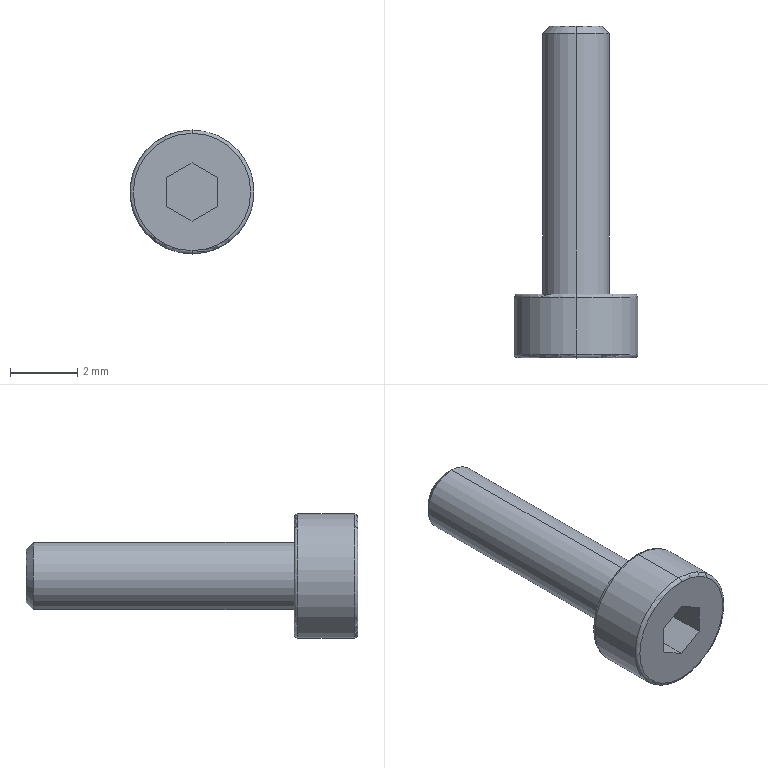Part | SolidWorks | features ICE 2, Extrusion 1, Fillet 1, StudWizard 1 | 1 solid | 20 faces | box 3.7 x 9.9 x 3.7 mm | volume 41.479 mm3 | plane 10 | torus 4 | cylinder 4 | cone 2 | commonest cylinder face diameters 2 x2 3.7 x2
STEP:
#1=CARTESIAN_POINT('',(0.,1.8,-1.85));
#2=VERTEX_POINT('',#1);
#3=CARTESIAN_POINT('',(0.,1.8,1.85));
#4=VERTEX_POINT('',#3);
#5=CARTESIAN_POINT('',(0.,1.8,0.));
#6=DIRECTION('',(0.,-1.,0.));
#7=DIRECTION('',(0.,0.,1.));
#8=AXIS2_PLACEMENT_3D('',#5,#6,#7);
#9=CIRCLE('',#8,1.85);
#10=EDGE_CURVE('',#2,#4,#9,.T.);
#11=ORIENTED_EDGE('',*,*,#10,.F.);
#12=CARTESIAN_POINT('',(0.,1.9,-1.75));
#13=VERTEX_POINT('',#12);
#14=CARTESIAN_POINT('',(0.,1.8,-1.75));
#15=DIRECTION('',(1.,0.,0.));
#16=DIRECTION('',(0.,0.,-1.));
#17=AXIS2_PLACEMENT_3D('',#14,#15,#16);
#18=CIRCLE('',#17,0.1);
#19=EDGE_CURVE('',#2,#13,#18,.T.);
#20=ORIENTED_EDGE('',*,*,#19,.T.);
#21=CARTESIAN_POINT('',(0.,1.9,1.75));
#22=VERTEX_POINT('',#21);
#23=CARTESIAN_POINT('',(0.,1.9,0.));
#24=DIRECTION('',(0.,1.,0.));
#25=DIRECTION('',(0.,0.,1.));
#26=AXIS2_PLACEMENT_3D('',#23,#24,#25);
#27=CIRCLE('',#26,1.75);
#28=EDGE_CURVE('',#22,#13,#27,.T.);
#29=ORIENTED_EDGE('',*,*,#28,.F.);
#30=CARTESIAN_POINT('',(0.,1.8,1.75));
#31=DIRECTION('',(-1.,0.,0.));
#32=DIRECTION('',(0.,0.,1.));
#33=AXIS2_PLACEMENT_3D('',#30,#31,#32);
#34=CIRCLE('',#33,0.1);
#35=EDGE_CURVE('',#4,#22,#34,.T.);
#36=ORIENTED_EDGE('',*,*,#35,.F.);
#37=EDGE_LOOP('',(#11,#20,#29,#36));
#38=FACE_OUTER_BOUND('',#37,.T.);
#39=CARTESIAN_POINT('',(0.,1.8,0.));
#40=DIRECTION('',(0.,1.,0.));
#41=DIRECTION('',(0.,0.,1.));
#42=AXIS2_PLACEMENT_3D('',#39,#40,#41);
#43=TOROIDAL_SURFACE('',#42,1.75,0.1);
#44=ADVANCED_FACE('',(#38),#43,.T.);
#45=CARTESIAN_POINT('',(0.,0.,-1.75));
#46=VERTEX_POINT('',#45);
#47=CARTESIAN_POINT('',(0.,0.,1.75));
#48=VERTEX_POINT('',#47);
#49=CARTESIAN_POINT('',(0.,0.,0.));
#50=DIRECTION('',(0.,-1.,0.));
#51=DIRECTION('',(0.,0.,1.));
#52=AXIS2_PLACEMENT_3D('',#49,#50,#51);
#53=CIRCLE('',#52,1.75);
#54=EDGE_CURVE('',#46,#48,#53,.T.);
#55=ORIENTED_EDGE('',*,*,#54,.F.);
#56=CARTESIAN_POINT('',(0.,0.1,-1.85));
#57=VERTEX_POINT('',#56);
#58=CARTESIAN_POINT('',(0.,0.1,-1.75));
#59=DIRECTION('',(1.,0.,0.));
#60=DIRECTION('',(0.,0.,-1.));
#61=AXIS2_PLACEMENT_3D('',#58,#59,#60);
#62=CIRCLE('',#61,0.1);
#63=EDGE_CURVE('',#46,#57,#62,.T.);
#64=ORIENTED_EDGE('',*,*,#63,.T.);
#65=CARTESIAN_POINT('',(0.,0.1,1.85));
#66=VERTEX_POINT('',#65);
#67=CARTESIAN_POINT('',(0.,0.1,0.));
#68=DIRECTION('',(0.,1.,0.));
#69=DIRECTION('',(0.,0.,1.));
#70=AXIS2_PLACEMENT_3D('',#67,#68,#69);
#71=CIRCLE('',#70,1.85);
#72=EDGE_CURVE('',#66,#57,#71,.T.);
#73=ORIENTED_EDGE('',*,*,#72,.F.);
#74=CARTESIAN_POINT('',(0.,0.1,1.75));
#75=DIRECTION('',(-1.,0.,0.));
#76=DIRECTION('',(0.,0.,1.));
#77=AXIS2_PLACEMENT_3D('',#74,#75,#76);
#78=CIRCLE('',#77,0.1);
#79=EDGE_CURVE('',#48,#66,#78,.T.);
#80=ORIENTED_EDGE('',*,*,#79,.F.);
#81=EDGE_LOOP('',(#55,#64,#73,#80));
#82=FACE_OUTER_BOUND('',#81,.T.);
#83=CARTESIAN_POINT('',(0.,0.1,0.));
#84=DIRECTION('',(0.,1.,0.));
#85=DIRECTION('',(0.,0.,1.));
#86=AXIS2_PLACEMENT_3D('',#83,#84,#85);
#87=TOROIDAL_SURFACE('',#86,1.75,0.1);
#88=ADVANCED_FACE('',(#82),#87,.T.);
#89=CARTESIAN_POINT('',(0.,9.9,-0.7835));
#90=VERTEX_POINT('',#89);
#91=CARTESIAN_POINT('',(0.,9.9,0.7835));
#92=VERTEX_POINT('',#91);
#93=CARTESIAN_POINT('',(0.,9.9,0.));
#94=DIRECTION('',(0.,-1.,0.));
#95=DIRECTION('',(0.,0.,-1.));
#96=AXIS2_PLACEMENT_3D('',#93,#94,#95);
#97=CIRCLE('',#96,0.7835);
#98=EDGE_CURVE('',#90,#92,#97,.T.);
#99=ORIENTED_EDGE('',*,*,#98,.T.);
#100=CARTESIAN_POINT('',(0.,9.684,1.));
#101=VERTEX_POINT('',#100);
#102=CARTESIAN_POINT('',(0.,9.684,1.));
#103=DIRECTION('',(0.,-0.7071,0.7071));
#104=VECTOR('',#103,1000.);
#105=LINE('',#102,#104);
#106=EDGE_CURVE('',#92,#101,#105,.T.);
#107=ORIENTED_EDGE('',*,*,#106,.T.);
#108=CARTESIAN_POINT('',(0.,9.684,-1.));
#109=VERTEX_POINT('',#108);
#110=CARTESIAN_POINT('',(0.,9.684,0.));
#111=DIRECTION('',(0.,-1.,0.));
#112=DIRECTION('',(0.,0.,-1.));
#113=AXIS2_PLACEMENT_3D('',#110,#111,#112);
#114=CIRCLE('',#113,1.);
#115=EDGE_CURVE('',#109,#101,#114,.T.);
#116=ORIENTED_EDGE('',*,*,#115,.F.);
#117=CARTESIAN_POINT('',(0.,9.684,-1.));
#118=DIRECTION('',(0.,-0.7071,-0.7071));
#119=VECTOR('',#118,1000.);
#120=LINE('',#117,#119);
#121=EDGE_CURVE('',#90,#109,#120,.T.);
#122=ORIENTED_EDGE('',*,*,#121,.F.);
#123=EDGE_LOOP('',(#99,#107,#116,#122));
#124=FACE_OUTER_BOUND('',#123,.T.);
#125=CARTESIAN_POINT('',(0.,9.684,0.));
#126=DIRECTION('',(0.,-1.,0.));
#127=DIRECTION('',(0.,0.,-1.));
#128=AXIS2_PLACEMENT_3D('',#125,#126,#127);
#129=CONICAL_SURFACE('',#128,1.,0.7854);
#130=ADVANCED_FACE('',(#124),#129,.T.);
#131=ORIENTED_EDGE('',*,*,#115,.T.);
#132=CARTESIAN_POINT('',(0.,1.9,1.));
#133=VERTEX_POINT('',#132);
#134=CARTESIAN_POINT('',(0.,6.72,1.));
#135=DIRECTION('',(0.,-1.,0.));
#136=VECTOR('',#135,1000.);
#137=LINE('',#134,#136);
#138=EDGE_CURVE('',#101,#133,#137,.T.);
#139=ORIENTED_EDGE('',*,*,#138,.T.);
#140=CARTESIAN_POINT('',(0.,1.9,-1.));
#141=VERTEX_POINT('',#140);
#142=CARTESIAN_POINT('',(0.,1.9,0.));
#143=DIRECTION('',(0.,1.,0.));
#144=DIRECTION('',(0.,0.,1.));
#145=AXIS2_PLACEMENT_3D('',#142,#143,#144);
#146=CIRCLE('',#145,1.);
#147=EDGE_CURVE('',#133,#141,#146,.T.);
#148=ORIENTED_EDGE('',*,*,#147,.T.);
#149=CARTESIAN_POINT('',(0.,6.72,-1.));
#150=DIRECTION('',(0.,-1.,0.));
#151=VECTOR('',#150,1000.);
#152=LINE('',#149,#151);
#153=EDGE_CURVE('',#109,#141,#152,.T.);
#154=ORIENTED_EDGE('',*,*,#153,.F.);
#155=EDGE_LOOP('',(#131,#139,#148,#154));
#156=FACE_OUTER_BOUND('',#155,.T.);
#157=CARTESIAN_POINT('',(0.,6.72,0.));
#158=DIRECTION('',(0.,-1.,0.));
#159=DIRECTION('',(0.,0.,-1.));
#160=AXIS2_PLACEMENT_3D('',#157,#158,#159);
#161=CYLINDRICAL_SURFACE('',#160,1.);
#162=ADVANCED_FACE('',(#156),#161,.T.);
#163=ORIENTED_EDGE('',*,*,#10,.T.);
#164=CARTESIAN_POINT('',(0.,1.9,1.85));
#165=DIRECTION('',(0.,-1.,0.));
#166=VECTOR('',#165,1000.);
#167=LINE('',#164,#166);
#168=EDGE_CURVE('',#4,#66,#167,.T.);
#169=ORIENTED_EDGE('',*,*,#168,.T.);
#170=ORIENTED_EDGE('',*,*,#72,.T.);
#171=CARTESIAN_POINT('',(0.,1.9,-1.85));
#172=DIRECTION('',(0.,-1.,0.));
#173=VECTOR('',#172,1000.);
#174=LINE('',#171,#173);
#175=EDGE_CURVE('',#2,#57,#174,.T.);
#176=ORIENTED_EDGE('',*,*,#175,.F.);
#177=EDGE_LOOP('',(#163,#169,#170,#176));
#178=FACE_OUTER_BOUND('',#177,.T.);
#179=CARTESIAN_POINT('',(0.,1.9,0.));
#180=DIRECTION('',(0.,-1.,0.));
#181=DIRECTION('',(0.,0.,-1.));
#182=AXIS2_PLACEMENT_3D('',#179,#180,#181);
#183=CYLINDRICAL_SURFACE('',#182,1.85);
#184=ADVANCED_FACE('',(#178),#183,.T.);
#185=ORIENTED_EDGE('',*,*,#168,.F.);
#186=CARTESIAN_POINT('',(0.,1.8,0.));
#187=DIRECTION('',(0.,-1.,0.));
#188=DIRECTION('',(0.,0.,1.));
#189=AXIS2_PLACEMENT_3D('',#186,#187,#188);
#190=CIRCLE('',#189,1.85);
#191=EDGE_CURVE('',#4,#2,#190,.T.);
#192=ORIENTED_EDGE('',*,*,#191,.T.);
#193=ORIENTED_EDGE('',*,*,#175,.T.);
#194=CARTESIAN_POINT('',(0.,0.1,0.));
#195=DIRECTION('',(0.,1.,0.));
#196=DIRECTION('',(0.,0.,1.));
#197=AXIS2_PLACEMENT_3D('',#194,#195,#196);
#198=CIRCLE('',#197,1.85);
#199=EDGE_CURVE('',#57,#66,#198,.T.);
#200=ORIENTED_EDGE('',*,*,#199,.T.);
#201=EDGE_LOOP('',(#185,#192,#193,#200));
#202=FACE_OUTER_BOUND('',#201,.T.);
#203=CARTESIAN_POINT('',(0.,1.9,0.));
#204=DIRECTION('',(0.,-1.,0.));
#205=DIRECTION('',(0.,0.,-1.));
#206=AXIS2_PLACEMENT_3D('',#203,#204,#205);
#207=CYLINDRICAL_SURFACE('',#206,1.85);
#208=ADVANCED_FACE('',(#202),#207,.T.);
#209=ORIENTED_EDGE('',*,*,#28,.T.);
#210=CARTESIAN_POINT('',(0.,1.9,0.));
#211=DIRECTION('',(0.,1.,0.));
#212=DIRECTION('',(0.,0.,1.));
#213=AXIS2_PLACEMENT_3D('',#210,#211,#212);
#214=CIRCLE('',#213,1.75);
#215=EDGE_CURVE('',#13,#22,#214,.T.);
#216=ORIENTED_EDGE('',*,*,#215,.T.);
#217=EDGE_LOOP('',(#209,#216));
#218=FACE_OUTER_BOUND('',#217,.T.);
#219=CARTESIAN_POINT('',(0.,1.9,0.));
#220=DIRECTION('',(0.,1.,0.));
#221=DIRECTION('',(0.,0.,1.));
#222=AXIS2_PLACEMENT_3D('',#219,#220,#221);
#223=CIRCLE('',#222,1.);
#224=EDGE_CURVE('',#141,#133,#223,.T.);
#225=ORIENTED_EDGE('',*,*,#224,.F.);
#226=ORIENTED_EDGE('',*,*,#147,.F.);
#227=EDGE_LOOP('',(#225,#226));
#228=FACE_BOUND('',#227,.T.);
#229=CARTESIAN_POINT('',(0.,1.9,0.));
#230=DIRECTION('',(0.,1.,0.));
#231=DIRECTION('',(0.,0.,1.));
#232=AXIS2_PLACEMENT_3D('',#229,#230,#231);
#233=PLANE('',#232);
#234=ADVANCED_FACE('',(#218,#228),#233,.T.);
#235=CARTESIAN_POINT('',(0.,0.,0.));
#236=DIRECTION('',(0.,-1.,0.));
#237=DIRECTION('',(0.,0.,1.));
#238=AXIS2_PLACEMENT_3D('',#235,#236,#237);
#239=CIRCLE('',#238,1.75);
#240=EDGE_CURVE('',#48,#46,#239,.T.);
#241=ORIENTED_EDGE('',*,*,#240,.T.);
#242=ORIENTED_EDGE('',*,*,#54,.T.);
#243=EDGE_LOOP('',(#241,#242));
#244=FACE_OUTER_BOUND('',#243,.T.);
#245=CARTESIAN_POINT('',(0.,0.,0.866));
#246=VERTEX_POINT('',#245);
#247=CARTESIAN_POINT('',(-0.75,0.,0.433));
#248=VERTEX_POINT('',#247);
#249=CARTESIAN_POINT('',(0.,0.,0.866));
#250=DIRECTION('',(-0.866,0.,-0.5));
#251=VECTOR('',#250,1000.);
#252=LINE('',#249,#251);
#253=EDGE_CURVE('',#246,#248,#252,.T.);
#254=ORIENTED_EDGE('',*,*,#253,.F.);
#255=CARTESIAN_POINT('',(0.75,0.,0.433));
#256=VERTEX_POINT('',#255);
#257=CARTESIAN_POINT('',(0.75,0.,0.433));
#258=DIRECTION('',(-0.866,0.,0.5));
#259=VECTOR('',#258,1000.);
#260=LINE('',#257,#259);
#261=EDGE_CURVE('',#256,#246,#260,.T.);
#262=ORIENTED_EDGE('',*,*,#261,.F.);
#263=CARTESIAN_POINT('',(0.75,0.,-0.433));
#264=VERTEX_POINT('',#263);
#265=CARTESIAN_POINT('',(0.75,0.,-0.433));
#266=DIRECTION('',(0.,0.,1.));
#267=VECTOR('',#266,1000.);
#268=LINE('',#265,#267);
#269=EDGE_CURVE('',#264,#256,#268,.T.);
#270=ORIENTED_EDGE('',*,*,#269,.F.);
#271=CARTESIAN_POINT('',(0.,0.,-0.866));
#272=VERTEX_POINT('',#271);
#273=CARTESIAN_POINT('',(0.,0.,-0.866));
#274=DIRECTION('',(0.866,0.,0.5));
#275=VECTOR('',#274,1000.);
#276=LINE('',#273,#275);
#277=EDGE_CURVE('',#272,#264,#276,.T.);
#278=ORIENTED_EDGE('',*,*,#277,.F.);
#279=CARTESIAN_POINT('',(-0.75,0.,-0.433));
#280=VERTEX_POINT('',#279);
#281=CARTESIAN_POINT('',(-0.75,0.,-0.433));
#282=DIRECTION('',(0.866,0.,-0.5));
#283=VECTOR('',#282,1000.);
#284=LINE('',#281,#283);
#285=EDGE_CURVE('',#280,#272,#284,.T.);
#286=ORIENTED_EDGE('',*,*,#285,.F.);
#287=CARTESIAN_POINT('',(-0.75,0.,0.433));
#288=DIRECTION('',(0.,0.,-1.));
#289=VECTOR('',#288,1000.);
#290=LINE('',#287,#289);
#291=EDGE_CURVE('',#248,#280,#290,.T.);
#292=ORIENTED_EDGE('',*,*,#291,.F.);
#293=EDGE_LOOP('',(#254,#262,#270,#278,#286,#292));
#294=FACE_BOUND('',#293,.T.);
#295=CARTESIAN_POINT('',(0.,0.,0.));
#296=DIRECTION('',(0.,1.,0.));
#297=DIRECTION('',(0.,0.,1.));
#298=AXIS2_PLACEMENT_3D('',#295,#296,#297);
#299=PLANE('',#298);
#300=ADVANCED_FACE('',(#244,#294),#299,.F.);
#301=ORIENTED_EDGE('',*,*,#138,.F.);
#302=CARTESIAN_POINT('',(0.,9.684,0.));
#303=DIRECTION('',(0.,-1.,0.));
#304=DIRECTION('',(0.,0.,-1.));
#305=AXIS2_PLACEMENT_3D('',#302,#303,#304);
#306=CIRCLE('',#305,1.);
#307=EDGE_CURVE('',#101,#109,#306,.T.);
#308=ORIENTED_EDGE('',*,*,#307,.T.);
#309=ORIENTED_EDGE('',*,*,#153,.T.);
#310=ORIENTED_EDGE('',*,*,#224,.T.);
#311=EDGE_LOOP('',(#301,#308,#309,#310));
#312=FACE_OUTER_BOUND('',#311,.T.);
#313=CARTESIAN_POINT('',(0.,6.72,0.));
#314=DIRECTION('',(0.,-1.,0.));
#315=DIRECTION('',(0.,0.,-1.));
#316=AXIS2_PLACEMENT_3D('',#313,#314,#315);
#317=CYLINDRICAL_SURFACE('',#316,1.);
#318=ADVANCED_FACE('',(#312),#317,.T.);
#319=ORIENTED_EDGE('',*,*,#98,.F.);
#320=CARTESIAN_POINT('',(0.,9.9,0.));
#321=DIRECTION('',(0.,-1.,0.));
#322=DIRECTION('',(0.,0.,-1.));
#323=AXIS2_PLACEMENT_3D('',#320,#321,#322);
#324=CIRCLE('',#323,0.7835);
#325=EDGE_CURVE('',#92,#90,#324,.T.);
#326=ORIENTED_EDGE('',*,*,#325,.F.);
#327=EDGE_LOOP('',(#319,#326));
#328=FACE_OUTER_BOUND('',#327,.T.);
#329=CARTESIAN_POINT('',(0.7835,9.9,0.));
#330=DIRECTION('',(0.,1.,0.));
#331=DIRECTION('',(0.,0.,1.));
#332=AXIS2_PLACEMENT_3D('',#329,#330,#331);
#333=PLANE('',#332);
#334=ADVANCED_FACE('',(#328),#333,.T.);
#335=ORIENTED_EDGE('',*,*,#106,.F.);
#336=ORIENTED_EDGE('',*,*,#325,.T.);
#337=ORIENTED_EDGE('',*,*,#121,.T.);
#338=ORIENTED_EDGE('',*,*,#307,.F.);
#339=EDGE_LOOP('',(#335,#336,#337,#338));
#340=FACE_OUTER_BOUND('',#339,.T.);
#341=CARTESIAN_POINT('',(0.,9.684,0.));
#342=DIRECTION('',(0.,-1.,0.));
#343=DIRECTION('',(0.,0.,-1.));
#344=AXIS2_PLACEMENT_3D('',#341,#342,#343);
#345=CONICAL_SURFACE('',#344,1.,0.7854);
#346=ADVANCED_FACE('',(#340),#345,.T.);
#347=ORIENTED_EDGE('',*,*,#261,.T.);
#348=CARTESIAN_POINT('',(0.,2.,0.866));
#349=VERTEX_POINT('',#348);
#350=CARTESIAN_POINT('',(0.,2.,0.866));
#351=DIRECTION('',(0.,-1.,0.));
#352=VECTOR('',#351,1000.);
#353=LINE('',#350,#352);
#354=EDGE_CURVE('',#349,#246,#353,.T.);
#355=ORIENTED_EDGE('',*,*,#354,.F.);
#356=CARTESIAN_POINT('',(0.75,2.,0.433));
#357=VERTEX_POINT('',#356);
#358=CARTESIAN_POINT('',(0.75,2.,0.433));
#359=DIRECTION('',(-0.866,0.,0.5));
#360=VECTOR('',#359,1000.);
#361=LINE('',#358,#360);
#362=EDGE_CURVE('',#357,#349,#361,.T.);
#363=ORIENTED_EDGE('',*,*,#362,.F.);
#364=CARTESIAN_POINT('',(0.75,2.,0.433));
#365=DIRECTION('',(0.,-1.,0.));
#366=VECTOR('',#365,1000.);
#367=LINE('',#364,#366);
#368=EDGE_CURVE('',#357,#256,#367,.T.);
#369=ORIENTED_EDGE('',*,*,#368,.T.);
#370=EDGE_LOOP('',(#347,#355,#363,#369));
#371=FACE_OUTER_BOUND('',#370,.T.);
#372=CARTESIAN_POINT('',(0.75,2.,0.433));
#373=DIRECTION('',(0.5,0.,0.866));
#374=DIRECTION('',(0.866,0.,-0.5));
#375=AXIS2_PLACEMENT_3D('',#372,#373,#374);
#376=PLANE('',#375);
#377=ADVANCED_FACE('',(#371),#376,.F.);
#378=ORIENTED_EDGE('',*,*,#269,.T.);
#379=ORIENTED_EDGE('',*,*,#368,.F.);
#380=CARTESIAN_POINT('',(0.75,2.,-0.433));
#381=VERTEX_POINT('',#380);
#382=CARTESIAN_POINT('',(0.75,2.,-0.433));
#383=DIRECTION('',(0.,0.,1.));
#384=VECTOR('',#383,1000.);
#385=LINE('',#382,#384);
#386=EDGE_CURVE('',#381,#357,#385,.T.);
#387=ORIENTED_EDGE('',*,*,#386,.F.);
#388=CARTESIAN_POINT('',(0.75,2.,-0.433));
#389=DIRECTION('',(0.,-1.,0.));
#390=VECTOR('',#389,1000.);
#391=LINE('',#388,#390);
#392=EDGE_CURVE('',#381,#264,#391,.T.);
#393=ORIENTED_EDGE('',*,*,#392,.T.);
#394=EDGE_LOOP('',(#378,#379,#387,#393));
#395=FACE_OUTER_BOUND('',#394,.T.);
#396=CARTESIAN_POINT('',(0.75,2.,-0.433));
#397=DIRECTION('',(1.,0.,0.));
#398=DIRECTION('',(0.,0.,-1.));
#399=AXIS2_PLACEMENT_3D('',#396,#397,#398);
#400=PLANE('',#399);
#401=ADVANCED_FACE('',(#395),#400,.F.);
#402=ORIENTED_EDGE('',*,*,#277,.T.);
#403=ORIENTED_EDGE('',*,*,#392,.F.);
#404=CARTESIAN_POINT('',(0.,2.,-0.866));
#405=VERTEX_POINT('',#404);
#406=CARTESIAN_POINT('',(0.,2.,-0.866));
#407=DIRECTION('',(0.866,0.,0.5));
#408=VECTOR('',#407,1000.);
#409=LINE('',#406,#408);
#410=EDGE_CURVE('',#405,#381,#409,.T.);
#411=ORIENTED_EDGE('',*,*,#410,.F.);
#412=CARTESIAN_POINT('',(0.,2.,-0.866));
#413=DIRECTION('',(0.,-1.,0.));
#414=VECTOR('',#413,1000.);
#415=LINE('',#412,#414);
#416=EDGE_CURVE('',#405,#272,#415,.T.);
#417=ORIENTED_EDGE('',*,*,#416,.T.);
#418=EDGE_LOOP('',(#402,#403,#411,#417));
#419=FACE_OUTER_BOUND('',#418,.T.);
#420=CARTESIAN_POINT('',(0.,2.,-0.866));
#421=DIRECTION('',(0.5,0.,-0.866));
#422=DIRECTION('',(-0.866,0.,-0.5));
#423=AXIS2_PLACEMENT_3D('',#420,#421,#422);
#424=PLANE('',#423);
#425=ADVANCED_FACE('',(#419),#424,.F.);
#426=ORIENTED_EDGE('',*,*,#285,.T.);
#427=ORIENTED_EDGE('',*,*,#416,.F.);
#428=CARTESIAN_POINT('',(-0.75,2.,-0.433));
#429=VERTEX_POINT('',#428);
#430=CARTESIAN_POINT('',(-0.75,2.,-0.433));
#431=DIRECTION('',(0.866,0.,-0.5));
#432=VECTOR('',#431,1000.);
#433=LINE('',#430,#432);
#434=EDGE_CURVE('',#429,#405,#433,.T.);
#435=ORIENTED_EDGE('',*,*,#434,.F.);
#436=CARTESIAN_POINT('',(-0.75,2.,-0.433));
#437=DIRECTION('',(0.,-1.,0.));
#438=VECTOR('',#437,1000.);
#439=LINE('',#436,#438);
#440=EDGE_CURVE('',#429,#280,#439,.T.);
#441=ORIENTED_EDGE('',*,*,#440,.T.);
#442=EDGE_LOOP('',(#426,#427,#435,#441));
#443=FACE_OUTER_BOUND('',#442,.T.);
#444=CARTESIAN_POINT('',(-0.75,2.,-0.433));
#445=DIRECTION('',(-0.5,0.,-0.866));
#446=DIRECTION('',(-0.866,0.,0.5));
#447=AXIS2_PLACEMENT_3D('',#444,#445,#446);
#448=PLANE('',#447);
#449=ADVANCED_FACE('',(#443),#448,.F.);
#450=ORIENTED_EDGE('',*,*,#291,.T.);
#451=ORIENTED_EDGE('',*,*,#440,.F.);
#452=CARTESIAN_POINT('',(-0.75,2.,0.433));
#453=VERTEX_POINT('',#452);
#454=CARTESIAN_POINT('',(-0.75,2.,0.433));
#455=DIRECTION('',(0.,0.,-1.));
#456=VECTOR('',#455,1000.);
#457=LINE('',#454,#456);
#458=EDGE_CURVE('',#453,#429,#457,.T.);
#459=ORIENTED_EDGE('',*,*,#458,.F.);
#460=CARTESIAN_POINT('',(-0.75,2.,0.433));
#461=DIRECTION('',(0.,-1.,0.));
#462=VECTOR('',#461,1000.);
#463=LINE('',#460,#462);
#464=EDGE_CURVE('',#453,#248,#463,.T.);
#465=ORIENTED_EDGE('',*,*,#464,.T.);
#466=EDGE_LOOP('',(#450,#451,#459,#465));
#467=FACE_OUTER_BOUND('',#466,.T.);
#468=CARTESIAN_POINT('',(-0.75,2.,0.433));
#469=DIRECTION('',(-1.,0.,0.));
#470=DIRECTION('',(0.,0.,1.));
#471=AXIS2_PLACEMENT_3D('',#468,#469,#470);
#472=PLANE('',#471);
#473=ADVANCED_FACE('',(#467),#472,.F.);
#474=ORIENTED_EDGE('',*,*,#253,.T.);
#475=ORIENTED_EDGE('',*,*,#464,.F.);
#476=CARTESIAN_POINT('',(0.,2.,0.866));
#477=DIRECTION('',(-0.866,0.,-0.5));
#478=VECTOR('',#477,1000.);
#479=LINE('',#476,#478);
#480=EDGE_CURVE('',#349,#453,#479,.T.);
#481=ORIENTED_EDGE('',*,*,#480,.F.);
#482=ORIENTED_EDGE('',*,*,#354,.T.);
#483=EDGE_LOOP('',(#474,#475,#481,#482));
#484=FACE_OUTER_BOUND('',#483,.T.);
#485=CARTESIAN_POINT('',(0.,2.,0.866));
#486=DIRECTION('',(-0.5,0.,0.866));
#487=DIRECTION('',(0.866,0.,0.5));
#488=AXIS2_PLACEMENT_3D('',#485,#486,#487);
#489=PLANE('',#488);
#490=ADVANCED_FACE('',(#484),#489,.F.);
#491=ORIENTED_EDGE('',*,*,#362,.T.);
#492=ORIENTED_EDGE('',*,*,#480,.T.);
#493=ORIENTED_EDGE('',*,*,#458,.T.);
#494=ORIENTED_EDGE('',*,*,#434,.T.);
#495=ORIENTED_EDGE('',*,*,#410,.T.);
#496=ORIENTED_EDGE('',*,*,#386,.T.);
#497=EDGE_LOOP('',(#491,#492,#493,#494,#495,#496));
#498=FACE_OUTER_BOUND('',#497,.T.);
#499=CARTESIAN_POINT('',(0.,2.,0.));
#500=DIRECTION('',(0.,-1.,0.));
#501=DIRECTION('',(0.,0.,-1.));
#502=AXIS2_PLACEMENT_3D('',#499,#500,#501);
#503=PLANE('',#502);
#504=ADVANCED_FACE('',(#498),#503,.T.);
#505=ORIENTED_EDGE('',*,*,#63,.F.);
#506=ORIENTED_EDGE('',*,*,#240,.F.);
#507=ORIENTED_EDGE('',*,*,#79,.T.);
#508=ORIENTED_EDGE('',*,*,#199,.F.);
#509=EDGE_LOOP('',(#505,#506,#507,#508));
#510=FACE_OUTER_BOUND('',#509,.T.);
#511=CARTESIAN_POINT('',(0.,0.1,0.));
#512=DIRECTION('',(0.,1.,0.));
#513=DIRECTION('',(0.,0.,1.));
#514=AXIS2_PLACEMENT_3D('',#511,#512,#513);
#515=TOROIDAL_SURFACE('',#514,1.75,0.1);
#516=ADVANCED_FACE('',(#510),#515,.T.);
#517=ORIENTED_EDGE('',*,*,#19,.F.);
#518=ORIENTED_EDGE('',*,*,#191,.F.);
#519=ORIENTED_EDGE('',*,*,#35,.T.);
#520=ORIENTED_EDGE('',*,*,#215,.F.);
#521=EDGE_LOOP('',(#517,#518,#519,#520));
#522=FACE_OUTER_BOUND('',#521,.T.);
#523=CARTESIAN_POINT('',(0.,1.8,0.));
#524=DIRECTION('',(0.,1.,0.));
#525=DIRECTION('',(0.,0.,1.));
#526=AXIS2_PLACEMENT_3D('',#523,#524,#525);
#527=TOROIDAL_SURFACE('',#526,1.75,0.1);
#528=ADVANCED_FACE('',(#522),#527,.T.);
#529=CLOSED_SHELL('',(#44,#88,#130,#162,#184,#208,#234,#300,#318,#334,#346,#377,#401,#425,#449,#473,#490,#504,#516,#528));
#530=MANIFOLD_SOLID_BREP('',#529);
#531=CARTESIAN_POINT('',(0.,0.,0.));
#532=DIRECTION('',(0.,0.,1.));
#533=DIRECTION('',(1.,0.,0.));
#534=AXIS2_PLACEMENT_3D('',#531,#532,#533);
#535=(LENGTH_UNIT()NAMED_UNIT(*)SI_UNIT(.MILLI.,.METRE.));
#536=UNCERTAINTY_MEASURE_WITH_UNIT(LENGTH_MEASURE(0.00001),#535,'','');
#537=(NAMED_UNIT(*)PLANE_ANGLE_UNIT()SI_UNIT($,.RADIAN.));
#538=(NAMED_UNIT(*)SI_UNIT($,.STERADIAN.)SOLID_ANGLE_UNIT());
#539=(GEOMETRIC_REPRESENTATION_CONTEXT(3)GLOBAL_UNCERTAINTY_ASSIGNED_CONTEXT((#536))GLOBAL_UNIT_ASSIGNED_CONTEXT((#535,#537,#538))REPRESENTATION_CONTEXT('',''));
#540=ADVANCED_BREP_SHAPE_REPRESENTATION('',(#530,#534),#539);